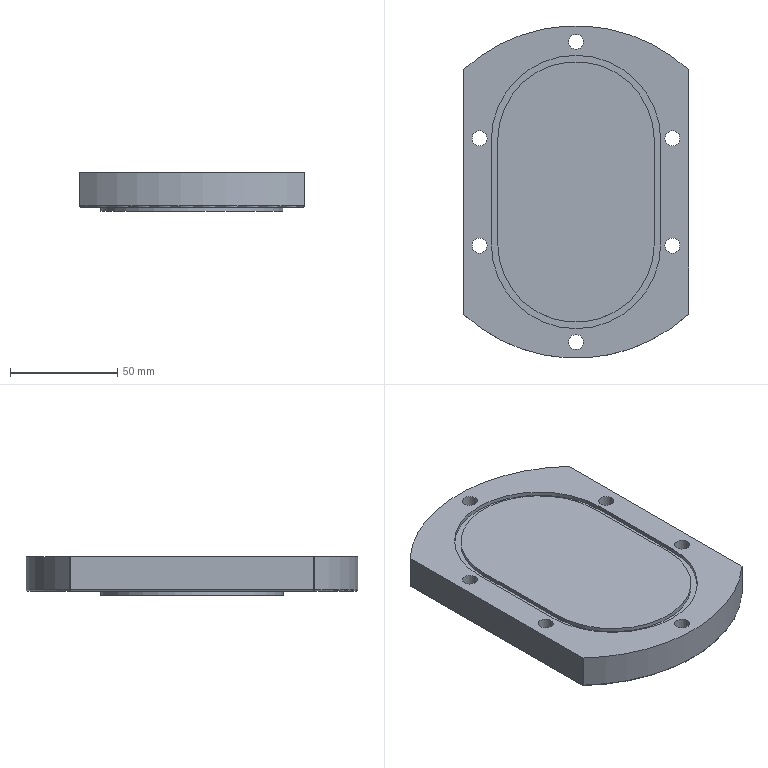NC program | NX | posted with a generic post | part box 105 x 155 x 18 mm
Whole program, first 1635 of 1782 lines:
N10 G17 G21 G94 G90
(FLOOR_WALL_COPY_1 , TOOL : D50)
N12 T02 M6
N14 G54
N16 G17 G0 G90 X-75.614 Y87.319 S1200 M3
N18 G43 Z30. H2
N20 Z7.65
N22 G94 G1 Z4.65 F1000.
N24 X-70.946
N26 X70.941 F2000.
N28 G2 X99.91 Y51.711 R112.241
N30 X101.323 Y48.895 R111.209
N32 X101.458 Y48.614 R111.395
N34 G1 X-101.459
N36 G3 X-109.633 Y25.245 R112.068
N38 X-110.453 Y21.379 R112.313
N40 X-112.069 Y9.909 R112.271
N42 G1 X112.07
N44 G2 X112.486 Y2.175 R112.313
N46 X112.5 Y1.294 R112.271
N48 G1 Y-1.294
N50 G2 X110.453 Y-21.377 R112.271
N52 X109.632 Y-25.245 R112.313
N54 X108.756 Y-28.795 R112.07
N56 G1 X-108.763
N58 G3 X-90.022 Y-67.5 R113.082
N60 G1 X90.002
N62 X93.727
N64 Z7.65
N66 G0 Z30.
N68 X-75.615 Y87.319
N70 Z7.3
N72 G1 Z4.3 F1000.
N74 X-70.946
N76 X70.942 F2000.
N78 G2 X88.734 Y69.167 R112.103
N80 X97.746 Y55.699 R112.241
N82 X101.46 Y48.614 R111.936
N84 G1 X-101.46
N86 G3 X-102.602 Y46.155 R110.938
N88 X-107.9 Y31.856 R112.068
N90 X-109.634 Y25.238 R110.735
N92 X-110.408 Y21.612 R112.347
N94 X-112.069 Y9.909 R112.313
N96 G1 X112.07
N98 G2 X112.5 Y1.291 R112.313
N100 G1 Y-1.284
N102 G2 X110.412 Y-21.592 R112.313
N104 X109.634 Y-25.238 R112.347
N106 X108.757 Y-28.795 R110.742
N108 G1 X-108.755
N110 G3 X-101.989 Y-47.492 R111.212
N112 X-98.21 Y-54.871 R111.831
N114 X-93.788 Y-62.135 R112.247
N116 X-90.007 Y-67.5 R112.235
N118 G1 X90.003
N120 X93.727
N122 Z7.3
N124 G0 Z30.
N126 X-75.621 Y87.319
N128 Z6.95
N130 G1 Z3.95 F1000.
N132 X-70.952
N134 X70.951 F2000.
N136 G2 X94.377 Y61.235 R111.958
N138 X101.461 Y48.614 R111.28
N140 G1 X-101.461
N142 G3 X-102.339 Y46.736 R111.642
N144 X-104.144 Y42.556 R110.938
N146 X-105.517 Y39.02 R111.642
N148 X-107.606 Y32.837 R110.925
N150 X-109.531 Y25.683 R110.735
N152 X-109.633 Y25.245 R110.925
N154 X-110.481 Y21.234 R112.352
N156 X-112.068 Y9.909 R112.347
N158 G1 X112.069
N160 G2 X112.5 Y1.217 R112.347
N162 G1 Y-1.212
N164 G2 X110.511 Y-21.078 R112.347
N166 X109.633 Y-25.245 R112.351
N168 X109.534 Y-25.671 R110.932
N170 X108.757 Y-28.795 R110.742
N172 G1 X-108.755
N174 G3 X-107.927 Y-31.763 R110.883
N176 X-102.013 Y-47.442 R111.831
N178 X-98.213 Y-54.866 R110.045
N180 X-90.014 Y-67.5 R112.024
N182 G1 X90.009
N184 X93.73
N186 Z6.95
N188 G0 Z30.
N190 X-75.629 Y87.319
N192 Z6.6
N194 G1 Z3.6 F1000.
N196 X-70.96
N198 X70.955 F2000.
N200 G2 X95.056 Y60.179 R111.788
N202 X101.461 Y48.614 R111.28
N204 G1 X-101.467
N206 G3 X-107.823 Y32.116 R111.531
N208 X-109.474 Y25.926 R110.925
N210 X-112.074 Y9.909 R112.101
N212 G1 X112.073
N214 G2 X112.5 Y1.638 R112.103
N216 G1 Y-1.65
N218 G2 X109.476 Y-25.921 R112.103
N220 X108.757 Y-28.795 R110.932
N222 G1 X-108.756
N224 G3 X-102.23 Y-46.972 R111.909
N226 X-98.213 Y-54.866 R110.045
N228 X-90.014 Y-67.5 R112.024
N230 G1 X90.011
N232 X93.731
N234 Z6.6
N236 G0 Z30.
N238 X-75.653 Y87.297
N240 Z6.25
N242 G1 Z3.25 F1000.
N244 X-70.986
N246 X70.981 F2000.
N248 G2 X93.922 Y61.939 R111.788
N250 X98.532 Y54.299 R110.498
N252 X101.468 Y48.598 R112.024
N254 G1 X-101.475
N256 G3 X-104.906 Y40.665 R111.531
N258 X-107.813 Y32.15 R111.134
N260 X-108.774 Y28.712 R111.531
N262 X-109.386 Y26.294 R112.101
N264 X-112.077 Y9.899 R112.004
N266 G1 X112.075
N268 G2 X112.5 Y1.781 R112.006
N270 G1 Y-1.798
N272 G2 X109.384 Y-26.302 R112.006
N274 X108.774 Y-28.712 R112.103
N276 G1 X108.751 Y-28.801
N278 X-108.755
N280 G3 X-101.738 Y-48.027 R111.459
N282 X-98.21 Y-54.872 R111.909
N284 G1 X-98.144 Y-54.99
N286 G3 X-92.27 Y-64.37 R109.794
N288 X-90.007 Y-67.5 R112.274
N290 G1 X90.011
N292 X93.731
N294 Z6.25
N296 G0 Z30.
N298 X-75.638 Y87.294
N300 Z5.9
N302 G1 Z2.9 F1000.
N304 X-70.971
N306 X70.971 F2000.
N308 G2 X85.956 Y72.586 R112.036
N310 X91.507 Y65.449 R112.37
N312 X99.844 Y51.84 R110.498
N314 X101.467 Y48.596 R111.457
N316 G1 X-101.474
N318 G3 X-108.753 Y28.792 R111.134
N320 X-109.187 Y27.106 R112.004
N322 X-112.078 Y9.897 R111.966
N324 G1 X112.076
N326 G2 X112.5 Y1.834 R111.968
N328 G1 Y-1.853
N330 G2 X109.189 Y-27.099 R111.968
N332 X108.75 Y-28.801 R112.006
N334 G1 X-108.755
N336 G3 X-90.006 Y-67.5 R113.109
N338 G1 X90.003
N340 X93.727
N342 Z5.9
N344 G0 Z30.
N346 X-75.632 Y87.301
N348 Z5.55
N350 G1 Z2.55 F1000.
N352 X-70.966
N354 X70.962 F2000.
N356 G2 X98.163 Y54.958 R112.284
N358 X99.878 Y51.773 R112.37
N360 X101.464 Y48.601 R111.357
N362 G1 X-101.47
N364 G3 X-107.634 Y32.745 R111.273
N366 X-109.35 Y26.445 R112.1
N368 X-112.078 Y9.9 R111.966
N370 G1 X112.076
N372 G2 X112.5 Y1.834 R111.968
N374 G1 Y-1.853
N376 G2 X109.35 Y-26.443 R111.968
N378 X108.754 Y-28.8 R112.102
N380 G1 X-108.762
N382 G3 X-90.006 Y-67.5 R112.72
N384 G1 X90.003
N386 X93.727
N388 Z5.55
N390 G0 Z30.
N392 X-75.631 Y87.302
N394 Z5.2
N396 G1 Z2.2 F1000.
N398 X-70.965
N400 X70.961 F2000.
N402 G2 X101.464 Y48.601 R112.412
N404 G1 X-101.472
N406 G3 X-107.864 Y31.977 R110.937
N408 X-109.348 Y26.452 R112.1
N410 X-112.079 Y9.901 R111.905
N412 G1 X112.077
N414 G2 X112.5 Y1.915 R111.908
N416 G1 Y-1.937
N418 G2 X109.349 Y-26.448 R111.908
N420 X108.754 Y-28.8 R112.102
N422 G1 X-108.762
N424 G3 X-101.44 Y-48.651 R111.402
N426 X-100.103 Y-51.337 R111.147
N428 X-99.926 Y-51.68 R111.402
N430 G1 X-98.201 Y-54.887
N432 G3 X-98.078 Y-55.108 R112.256
N434 X-90.006 Y-67.5 R112.252
N436 G1 X90.002
N438 X93.727
N440 Z5.2
N442 G0 Z30.
N444 X-75.632 Y87.302
N446 Z4.85
N448 G1 Z1.85 F1000.
N450 X-70.965
N452 X70.961 F2000.
N454 G2 X98.468 Y54.41 R112.27
N456 X99.921 Y51.69 R112.297
N458 X101.325 Y48.889 R111.102
N460 X101.464 Y48.601 R111.145
N462 G1 X-101.472
N464 G3 X-107.772 Y32.289 R110.937
N466 X-109.377 Y26.333 R112.065
N468 X-112.079 Y9.901 R111.905
N470 G1 X112.077
N472 G2 X112.5 Y1.915 R111.908
N474 G1 Y-1.937
N476 G2 X109.378 Y-26.329 R111.908
N478 X108.755 Y-28.8 R112.067
N480 G1 X-108.756
N482 G3 X-90.007 Y-67.5 R112.605
N484 G1 X90.002
N486 X93.727
N488 Z4.85
N490 G0 Z30.
N492 X-75.615 Y87.319
N494 Z4.5
N496 G1 Z1.5 F1000.
N498 X-70.947
N500 X70.942 F2000.
N502 G2 X92.898 Y63.46 R112.082
N504 X97.478 Y56.165 R112.297
N506 X101.46 Y48.614 R111.937
N508 G1 X-101.459
N510 G3 X-108.239 Y30.685 R112.065
N512 X-109.635 Y25.237 R112.103
N514 X-110.409 Y21.604 R112.345
N516 X-112.069 Y9.909 R112.311
N518 G1 X112.07
N520 G2 X112.5 Y1.296 R112.311
N522 G1 Y-1.288
N524 G2 X110.409 Y-21.605 R112.311
N526 X109.635 Y-25.237 R112.346
N528 X108.756 Y-28.795 R112.105
N530 G1 X-108.755
N532 G3 X-101.856 Y-47.777 R111.107
N534 X-98.21 Y-54.872 R111.838
N536 X-93.852 Y-62.039 R112.245
N538 X-90.007 Y-67.5 R112.234
N540 G1 X90.003
N542 X93.727
N544 Z4.5
N546 G0 Z30.
N548 X-75.621 Y87.319
N550 Z4.15
N552 G1 Z1.15 F1000.
N554 X-70.952
N556 X70.95 F2000.
N558 G2 X94.377 Y61.236 R111.982
N560 X101.461 Y48.614 R111.309
N562 G1 X-101.46
N564 G3 X-102.512 Y46.353 R111.74
N566 X-107.911 Y31.819 R112.103
N568 X-109.633 Y25.244 R110.994
N570 X-110.47 Y21.29 R112.352
N572 X-112.068 Y9.909 R112.346
N574 G1 X112.069
N576 G2 X112.5 Y1.22 R112.346
N578 G1 Y-1.214
N580 G2 X110.505 Y-21.112 R112.346
N582 X109.633 Y-25.244 R112.351
N584 X108.756 Y-28.795 R111.001
N586 G1 X-108.755
N588 G3 X-107.859 Y-31.994 R110.902
N590 X-102.027 Y-47.411 R111.838
N592 X-98.213 Y-54.867 R110.088
N594 X-90.014 Y-67.5 R112.029
N596 G1 X90.009
N598 X93.73
N600 Z4.15
N602 G0 Z30.
N604 X-75.621 Y87.319
N606 Z3.8
N608 G1 Z0.8 F1000.
N610 X-70.952
N612 X70.95 F2000.
N614 G2 X93.525 Y62.532 R111.982
N616 X94.878 Y60.458 R112.368
N618 X101.461 Y48.614 R111.309
N620 G1 X-101.463
N622 G3 X-104.199 Y42.422 R111.661
N624 X-105.527 Y38.993 R111.74
N626 X-107.477 Y33.254 R110.994
N628 X-112.076 Y9.909 R112.194
N630 G1 X112.073
N632 G2 X112.5 Y1.68 R112.195
N634 G1 Y-1.718
N636 G2 X108.76 Y-28.795 R112.195
N638 G1 X-108.757
N640 G3 X-102.086 Y-47.284 R111.642
N642 X-98.213 Y-54.867 R110.088
N644 X-90.014 Y-67.5 R112.029
N646 G1 X90.009
N648 X93.73
N650 Z3.8
N652 G0 Z30.
N654 X-75.644 Y87.297
N656 Z3.45
N658 G1 Z0.45 F1000.
N660 X-70.973
N662 X70.981 F2000.
N664 G2 X88.117 Y69.95 R111.495
N666 X92.269 Y64.372 R112.368
N668 X99.593 Y52.321 R110.523
N670 X99.795 Y51.936 R112.368
N672 X101.466 Y48.598 R111.644
N674 G1 X-101.476
N676 G3 X-107.724 Y32.448 R111.462
N678 X-112.077 Y9.899 R112.194
N680 G1 X112.075
N682 G2 X112.5 Y1.771 R112.018
N684 G1 Y-1.788
N686 G2 X112.204 Y-8.333 R112.018
N688 X108.758 Y-28.801 R112.195
N690 G1 X-108.755
N692 G3 X-90.007 Y-67.5 R112.76
N694 G1 X90.011
N696 X93.731
N698 Z3.45
N700 G0 Z30.
N702 X-75.649 Y87.293
N704 Z3.1
N706 G1 Z0.1 F1000.
N708 X-70.978
N710 X70.986 F2000.
N712 G2 X88.748 Y69.145 R111.495
N714 X91.643 Y65.258 R112.395
N716 X99.837 Y51.853 R110.523
N718 X101.467 Y48.595 R111.474
N720 G1 X-101.477
N722 G3 X-108.761 Y28.76 R111.462
N724 X-109.934 Y23.91 R112.015
N726 X-112.078 Y9.896 R111.977
N728 G1 X112.076
N730 G2 X112.5 Y1.819 R111.979
N732 G1 Y-1.837
N734 G2 X109.904 Y-24.051 R111.979
N736 X108.75 Y-28.802 R112.018
N738 G1 X-108.755
N740 G3 X-90.006 Y-67.5 R113.105
N742 G1 X90.011
N744 X93.731
N746 Z3.1
N748 G0 Z30.
(FLOOR_WALL_COPY_COPY , TOOL : D50)
N750 X-75.612 Y87.319 S2500
N752 Z3.
N754 G1 Z0. F1000.
N756 X-70.944
N758 X70.94
N760 G2 X99.927 Y51.677 R112.283
N762 X101.311 Y48.918 R111.144
N764 X101.458 Y48.614 R111.395
N766 G1 X-101.459
N768 G3 X-109.634 Y25.24 R112.055
N770 X-112.077 Y9.909 R111.876
N772 G1 X112.076
N774 G2 X112.5 Y1.904 R111.879
N776 G1 Y-1.918
N778 G2 X109.634 Y-25.24 R111.879
N780 X108.756 Y-28.795 R112.057
N782 G1 X-108.763
N784 G3 X-90.022 Y-67.5 R113.084
N786 G1 X90.002
N788 X93.727
N790 Z3.
N792 G0 Z30.
N794 M5
(DRILLING , TOOL : ZXZ)
N796 T01 M6
N798 G54
N800 G17 G0 G90 X70. Y0. S5000 M3
N802 G43 Z30. H1
N804 G94 G81 G98 Z-1. F250. R3.
N806 X25. Y-45.
N808 X-25.
N810 X-70. Y0.
N812 X-25. Y45.
N814 X25.
N816 G80
N818 G0 X25. Y45. Z30.
N820 M5
(DRILLING_COPY , TOOL : 7.0ZT)
N822 T09 M6
N824 G54
N826 G17 G0 G90 X70. Y0. S2000 M3
N828 G43 Z30. H9
N830 G94 G83 G98 Z-21.103 F200. Q2. R3.
N832 X25. Y-45.
N834 Y45.
N836 X-25.
N838 Y-45.
N840 X-70. Y0.
N842 G80
N844 G0 X-70. Y0. Z30.
N846 M5
(PLANAR_PROFILE , TOOL : D3)
N848 T03 M6
N850 G54
N852 G17 G0 G90 X0. Y38. S5000 M3
N854 G43 Z30. H3
N856 Z3.
N858 G94 G1 Z-0.05 F500.
N860 X-24.25 F1100.
N862 G3 X-62.25 Y0. R38.
N864 X-24.25 Y-38. R38.
N866 G1 X24.25
N868 G3 X62.25 Y0. R38.
N870 X24.25 Y38. R38.
N872 G1 X0.
N874 Z2.95
N876 Z-0.1 F500.
N878 X24.25 F1100.
N880 G2 X62.25 Y0. R38.
N882 X24.25 Y-38. R38.
N884 G1 X-24.25
N886 G2 X-62.25 Y0. R38.
N888 X-24.25 Y38. R38.
N890 G1 X0.
N892 Z2.9
N894 Z-0.15 F500.
N896 X-24.25 F1100.
N898 G3 X-62.25 Y0. R38.
N900 X-24.25 Y-38. R38.
N902 G1 X24.25
N904 G3 X62.25 Y0. R38.
N906 X24.25 Y38. R38.
N908 G1 X0.
N910 Z2.85
N912 Z-0.2 F500.
N914 X24.25 F1100.
N916 G2 X62.25 Y0. R38.
N918 X24.25 Y-38. R38.
N920 G1 X-24.25
N922 G2 X-62.25 Y0. R38.
N924 X-24.25 Y38. R38.
N926 G1 X0.
N928 Z2.8
N930 Z-0.25 F500.
N932 X-24.25 F1100.
N934 G3 X-62.25 Y0. R38.
N936 X-24.25 Y-38. R38.
N938 G1 X24.25
N940 G3 X62.25 Y0. R38.
N942 X24.25 Y38. R38.
N944 G1 X0.
N946 Z2.75
N948 Z-0.3 F500.
N950 X24.25 F1100.
N952 G2 X62.25 Y0. R38.
N954 X24.25 Y-38. R38.
N956 G1 X-24.25
N958 G2 X-62.25 Y0. R38.
N960 X-24.25 Y38. R38.
N962 G1 X0.
N964 Z2.7
N966 Z-0.35 F500.
N968 X-24.25 F1100.
N970 G3 X-62.25 Y0. R38.
N972 X-24.25 Y-38. R38.
N974 G1 X24.25
N976 G3 X62.25 Y0. R38.
N978 X24.25 Y38. R38.
N980 G1 X0.
N982 Z2.65
N984 Z-0.4 F500.
N986 X24.25 F1100.
N988 G2 X62.25 Y0. R38.
N990 X24.25 Y-38. R38.
N992 G1 X-24.25
N994 G2 X-62.25 Y0. R38.
N996 X-24.25 Y38. R38.
N998 G1 X0.
N1000 Z2.6
N1002 Z-0.45 F500.
N1004 X-24.25 F1100.
N1006 G3 X-62.25 Y0. R38.
N1008 X-24.25 Y-38. R38.
N1010 G1 X24.25
N1012 G3 X62.25 Y0. R38.
N1014 X24.25 Y38. R38.
N1016 G1 X0.
N1018 Z2.55
N1020 Z-0.5 F500.
N1022 X24.25 F1100.
N1024 G2 X62.25 Y0. R38.
N1026 X24.25 Y-38. R38.
N1028 G1 X-24.25
N1030 G2 X-62.25 Y0. R38.
N1032 X-24.25 Y38. R38.
N1034 G1 X0.
N1036 Z2.5
N1038 Z-0.55 F500.
N1040 X-24.25 F1100.
N1042 G3 X-62.25 Y0. R38.
N1044 X-24.25 Y-38. R38.
N1046 G1 X24.25
N1048 G3 X62.25 Y0. R38.
N1050 X24.25 Y38. R38.
N1052 G1 X0.
N1054 Z2.45
N1056 Z-0.6 F500.
N1058 X24.25 F1100.
N1060 G2 X62.25 Y0. R38.
N1062 X24.25 Y-38. R38.
N1064 G1 X-24.25
N1066 G2 X-62.25 Y0. R38.
N1068 X-24.25 Y38. R38.
N1070 G1 X0.
N1072 Z2.4
N1074 Z-0.65 F500.
N1076 X-24.25 F1100.
N1078 G3 X-62.25 Y0. R38.
N1080 X-24.25 Y-38. R38.
N1082 G1 X24.25
N1084 G3 X62.25 Y0. R38.
N1086 X24.25 Y38. R38.
N1088 G1 X0.
N1090 Z2.35
N1092 Z-0.7 F500.
N1094 X24.25 F1100.
N1096 G2 X62.25 Y0. R38.
N1098 X24.25 Y-38. R38.
N1100 G1 X-24.25
N1102 G2 X-62.25 Y0. R38.
N1104 X-24.25 Y38. R38.
N1106 G1 X0.
N1108 Z2.3
N1110 Z-0.75 F500.
N1112 X-24.25 F1100.
N1114 G3 X-62.25 Y0. R38.
N1116 X-24.25 Y-38. R38.
N1118 G1 X24.25
N1120 G3 X62.25 Y0. R38.
N1122 X24.25 Y38. R38.
N1124 G1 X0.
N1126 Z2.25
N1128 Z-0.8 F500.
N1130 X24.25 F1100.
N1132 G2 X62.25 Y0. R38.
N1134 X24.25 Y-38. R38.
N1136 G1 X-24.25
N1138 G2 X-62.25 Y0. R38.
N1140 X-24.25 Y38. R38.
N1142 G1 X0.
N1144 Z2.2
N1146 Z-0.85 F500.
N1148 X-24.25 F1100.
N1150 G3 X-62.25 Y0. R38.
N1152 X-24.25 Y-38. R38.
N1154 G1 X24.25
N1156 G3 X62.25 Y0. R38.
N1158 X24.25 Y38. R38.
N1160 G1 X0.
N1162 Z2.15
N1164 Z-0.9 F500.
N1166 X24.25 F1100.
N1168 G2 X62.25 Y0. R38.
N1170 X24.25 Y-38. R38.
N1172 G1 X-24.25
N1174 G2 X-62.25 Y0. R38.
N1176 X-24.25 Y38. R38.
N1178 G1 X0.
N1180 Z2.1
N1182 Z-0.95 F500.
N1184 X-24.25 F1100.
N1186 G3 X-62.25 Y0. R38.
N1188 X-24.25 Y-38. R38.
N1190 G1 X24.25
N1192 G3 X62.25 Y0. R38.
N1194 X24.25 Y38. R38.
N1196 G1 X0.
N1198 Z2.05
N1200 Z-1. F500.
N1202 X24.25 F1100.
N1204 G2 X62.25 Y0. R38.
N1206 X24.25 Y-38. R38.
N1208 G1 X-24.25
N1210 G2 X-62.25 Y0. R38.
N1212 X-24.25 Y38. R38.
N1214 G1 X0.
N1216 Z2.
N1218 Z-1.05 F500.
N1220 X-24.25 F1100.
N1222 G3 X-62.25 Y0. R38.
N1224 X-24.25 Y-38. R38.
N1226 G1 X24.25
N1228 G3 X62.25 Y0. R38.
N1230 X24.25 Y38. R38.
N1232 G1 X0.
N1234 Z1.95
N1236 Z-1.1 F500.
N1238 X24.25 F1100.
N1240 G2 X62.25 Y0. R38.
N1242 X24.25 Y-38. R38.
N1244 G1 X-24.25
N1246 G2 X-62.25 Y0. R38.
N1248 X-24.25 Y38. R38.
N1250 G1 X0.
N1252 Z1.9
N1254 Z-1.15 F500.
N1256 X-24.25 F1100.
N1258 G3 X-62.25 Y0. R38.
N1260 X-24.25 Y-38. R38.
N1262 G1 X24.25
N1264 G3 X62.25 Y0. R38.
N1266 X24.25 Y38. R38.
N1268 G1 X0.
N1270 Z1.85
N1272 Z-1.2 F500.
N1274 X24.25 F1100.
N1276 G2 X62.25 Y0. R38.
N1278 X24.25 Y-38. R38.
N1280 G1 X-24.25
N1282 G2 X-62.25 Y0. R38.
N1284 X-24.25 Y38. R38.
N1286 G1 X0.
N1288 Z1.8
N1290 Z-1.25 F500.
N1292 X-24.25 F1100.
N1294 G3 X-62.25 Y0. R38.
N1296 X-24.25 Y-38. R38.
N1298 G1 X24.25
N1300 G3 X62.25 Y0. R38.
N1302 X24.25 Y38. R38.
N1304 G1 X0.
N1306 Z1.75
N1308 Z-1.3 F500.
N1310 X24.25 F1100.
N1312 G2 X62.25 Y0. R38.
N1314 X24.25 Y-38. R38.
N1316 G1 X-24.25
N1318 G2 X-62.25 Y0. R38.
N1320 X-24.25 Y38. R38.
N1322 G1 X0.
N1324 Z1.7
N1326 Z-1.35 F500.
N1328 X-24.25 F1100.
N1330 G3 X-62.25 Y0. R38.
N1332 X-24.25 Y-38. R38.
N1334 G1 X24.25
N1336 G3 X62.25 Y0. R38.
N1338 X24.25 Y38. R38.
N1340 G1 X0.
N1342 Z1.65
N1344 Z-1.4 F500.
N1346 X24.25 F1100.
N1348 G2 X62.25 Y0. R38.
N1350 X24.25 Y-38. R38.
N1352 G1 X-24.25
N1354 G2 X-62.25 Y0. R38.
N1356 X-24.25 Y38. R38.
N1358 G1 X0.
N1360 Z1.6
N1362 Z-1.45 F500.
N1364 X-24.25 F1100.
N1366 G3 X-62.25 Y0. R38.
N1368 X-24.25 Y-38. R38.
N1370 G1 X24.25
N1372 G3 X62.25 Y0. R38.
N1374 X24.25 Y38. R38.
N1376 G1 X0.
N1378 Z1.55
N1380 Z-1.5 F500.
N1382 X24.25 F1100.
N1384 G2 X62.25 Y0. R38.
N1386 X24.25 Y-38. R38.
N1388 G1 X-24.25
N1390 G2 X-62.25 Y0. R38.
N1392 X-24.25 Y38. R38.
N1394 G1 X0.
N1396 Z1.5
N1398 Z-1.55 F500.
N1400 X-24.25 F1100.
N1402 G3 X-62.25 Y0. R38.
N1404 X-24.25 Y-38. R38.
N1406 G1 X24.25
N1408 G3 X62.25 Y0. R38.
N1410 X24.25 Y38. R38.
N1412 G1 X0.
N1414 Z1.45
N1416 Z-1.6 F500.
N1418 X24.25 F1100.
N1420 G2 X62.25 Y0. R38.
N1422 X24.25 Y-38. R38.
N1424 G1 X-24.25
N1426 G2 X-62.25 Y0. R38.
N1428 X-24.25 Y38. R38.
N1430 G1 X0.
N1432 Z1.4
N1434 Z-1.65 F500.
N1436 X-24.25 F1100.
N1438 G3 X-62.25 Y0. R38.
N1440 X-24.25 Y-38. R38.
N1442 G1 X24.25
N1444 G3 X62.25 Y0. R38.
N1446 X24.25 Y38. R38.
N1448 G1 X0.
N1450 Z1.35
N1452 Z-1.7 F500.
N1454 X24.25 F1100.
N1456 G2 X62.25 Y0. R38.
N1458 X24.25 Y-38. R38.
N1460 G1 X-24.25
N1462 G2 X-62.25 Y0. R38.
N1464 X-24.25 Y38. R38.
N1466 G1 X0.
N1468 Z1.3
N1470 Z-1.75 F500.
N1472 X-24.25 F1100.
N1474 G3 X-62.25 Y0. R38.
N1476 X-24.25 Y-38. R38.
N1478 G1 X24.25
N1480 G3 X62.25 Y0. R38.
N1482 X24.25 Y38. R38.
N1484 G1 X0.
N1486 Z1.25
N1488 Z-1.8 F500.
N1490 X24.25 F1100.
N1492 G2 X62.25 Y0. R38.
N1494 X24.25 Y-38. R38.
N1496 G1 X-24.25
N1498 G2 X-62.25 Y0. R38.
N1500 X-24.25 Y38. R38.
N1502 G1 X0.
N1504 Z1.2
N1506 G0 Z30.
N1508 M5
(ZLEVEL_PROFILE_COPY , TOOL : D25R0.5)
N1510 T05 M6
N1512 G54
N1514 G17 G0 G90 X-65.122 Y74.248 S2000 M3
N1516 G43 Z30. H5
N1518 Z-0.348
N1520 G94 G1 X-60.623 Y66.405 F1000.
N1522 G3 X-58.461 Y65.149 R2.5
N1524 G1 X-57.852 Y65.147 F2200.
N1526 X-56.741 Y65.15
N1528 X56.81 Y65.149
N1530 X57.852 Y65.147
N1532 X58.461 Y65.149
N1534 G3 X60.623 Y66.405 R2.5
N1536 G1 X65.122 Y74.248
N1538 X-65.09 Y74.257 Z-0.696
N1540 X-60.619 Y66.411 F1000.
N1542 G3 X-58.461 Y65.149 R2.5
N1544 G1 X-57.243 Y65.142 F2200.
N1546 G2 X-56.789 Y65.15 R13.15
N1548 G1 X56.831
N1550 G2 X57.243 Y65.142 R13.15
N1552 G1 X58.461 Y65.149
N1554 G3 X60.619 Y66.411 R2.5
N1556 G1 X65.09 Y74.257
N1558 X-65.09 Z-1.043
N1560 X-60.619 Y66.411 F1000.
N1562 G3 X-58.461 Y65.149 R2.5
N1564 G1 X-57.243 Y65.142 F2200.
N1566 G2 X-56.789 Y65.15 R13.15
N1568 G1 X56.831
N1570 G2 X57.243 Y65.142 R13.15
N1572 G1 X58.461 Y65.149
N1574 G3 X60.619 Y66.411 R2.5
N1576 G1 X65.09 Y74.257
N1578 X-65.09 Z-1.391
N1580 X-60.619 Y66.411 F1000.
N1582 G3 X-58.461 Y65.149 R2.5
N1584 G1 X-57.243 Y65.142 F2200.
N1586 G2 X-56.789 Y65.15 R13.15
N1588 G1 X56.831
N1590 G2 X57.243 Y65.142 R13.15
N1592 G1 X58.461 Y65.149
N1594 G3 X60.619 Y66.411 R2.5
N1596 G1 X65.09 Y74.257
N1598 X-65.09 Z-1.739
N1600 X-60.619 Y66.411 F1000.
N1602 G3 X-58.461 Y65.149 R2.5
N1604 G1 X-57.243 Y65.142 F2200.
N1606 G2 X-56.789 Y65.15 R13.15
N1608 G1 X56.831
N1610 G2 X57.243 Y65.142 R13.15
N1612 G1 X58.461 Y65.149
N1614 G3 X60.619 Y66.411 R2.5
N1616 G1 X65.09 Y74.257
N1618 X-65.089 Z-2.087
N1620 X-60.619 Y66.411 F1000.
N1622 G3 X-58.461 Y65.149 R2.5
N1624 G1 X-57.243 Y65.142 F2200.
N1626 G2 X-56.789 Y65.15 R13.15
N1628 G1 X56.831
N1630 G2 X57.243 Y65.142 R13.15
N1632 G1 X58.461 Y65.149
N1634 G3 X60.619 Y66.411 R2.5
N1636 G1 X65.089 Y74.257
N1638 X-65.089 Z-2.435
N1640 X-60.619 Y66.412 F1000.
N1642 G3 X-58.461 Y65.149 R2.5
N1644 G1 X-57.243 Y65.142 F2200.
N1646 G2 X-56.789 Y65.15 R13.15
N1648 G1 X56.831
N1650 G2 X57.243 Y65.142 R13.15
N1652 G1 X58.461 Y65.149
N1654 G3 X60.619 Y66.412 R2.5
N1656 G1 X65.089 Y74.257
N1658 X-65.089 Z-2.783
N1660 X-60.619 Y66.412 F1000.
N1662 G3 X-58.461 Y65.149 R2.5
N1664 G1 X-57.243 Y65.142 F2200.
N1666 G2 X-56.789 Y65.15 R13.15
N1668 G1 X56.831
N1670 G2 X57.243 Y65.142 R13.15
N1672 G1 X58.461 Y65.149
N1674 G3 X60.619 Y66.412 R2.5
N1676 G1 X65.089 Y74.257
N1678 X-65.089 Z-3.13
N1680 X-60.619 Y66.412 F1000.
N1682 G3 X-58.461 Y65.149 R2.5
N1684 G1 X-57.243 Y65.142 F2200.
N1686 G2 X-56.789 Y65.15 R13.15
N1688 G1 X56.831
N1690 G2 X57.243 Y65.142 R13.15
N1692 G1 X58.461 Y65.149
N1694 G3 X60.619 Y66.412 R2.5
N1696 G1 X65.089 Y74.257
N1698 X-65.089 Y74.258 Z-3.478
N1700 X-60.619 Y66.412 F1000.
N1702 G3 X-58.461 Y65.149 R2.5
N1704 G1 X-57.243 Y65.142 F2200.
N1706 G2 X-56.789 Y65.15 R13.15
N1708 G1 X56.831
N1710 G2 X57.243 Y65.142 R13.15
N1712 G1 X58.461 Y65.149
N1714 G3 X60.619 Y66.412 R2.5
N1716 G1 X65.089 Y74.258
N1718 X-65.089 Z-3.826
N1720 X-60.619 Y66.412 F1000.
N1722 G3 X-58.461 Y65.149 R2.5
N1724 G1 X-57.243 Y65.142 F2200.
N1726 G2 X-56.789 Y65.15 R13.15
N1728 G1 X56.831
N1730 G2 X57.243 Y65.142 R13.15
N1732 G1 X58.461 Y65.149
N1734 G3 X60.619 Y66.412 R2.5
N1736 G1 X65.089 Y74.258
N1738 X-65.089 Z-4.174
N1740 X-60.619 Y66.412 F1000.
N1742 G3 X-58.461 Y65.149 R2.5
N1744 G1 X-57.243 Y65.142 F2200.
N1746 G2 X-56.789 Y65.15 R13.15
N1748 G1 X56.831
N1750 G2 X57.243 Y65.142 R13.15
N1752 G1 X58.461 Y65.149
N1754 G3 X60.619 Y66.412 R2.5
N1756 G1 X65.089 Y74.258
N1758 X-65.089 Z-4.522
N1760 X-60.619 Y66.412 F1000.
N1762 G3 X-58.461 Y65.149 R2.5
N1764 G1 X-57.243 Y65.142 F2200.
N1766 G2 X-56.789 Y65.15 R13.15
N1768 G1 X56.831
N1770 G2 X57.243 Y65.142 R13.15
N1772 G1 X58.461 Y65.149
N1774 G3 X60.619 Y66.412 R2.5
N1776 G1 X65.089 Y74.258
N1778 X-65.088 Z-4.87
N1780 X-60.619 Y66.412 F1000.
N1782 G3 X-58.461 Y65.149 R2.5
N1784 G1 X-57.243 Y65.142 F2200.
N1786 G2 X-56.789 Y65.15 R13.15
N1788 G1 X56.831
N1790 G2 X57.243 Y65.142 R13.15
N1792 G1 X58.461 Y65.149
N1794 G3 X60.619 Y66.412 R2.5
N1796 G1 X65.088 Y74.258
N1798 X-65.088 Z-5.217
N1800 X-60.619 Y66.412 F1000.
N1802 G3 X-58.461 Y65.149 R2.5
N1804 G1 X-57.243 Y65.142 F2200.
N1806 G2 X-56.789 Y65.15 R13.15
N1808 G1 X56.831
N1810 G2 X57.243 Y65.142 R13.15
N1812 G1 X58.461 Y65.149
N1814 G3 X60.619 Y66.412 R2.5
N1816 G1 X65.088 Y74.258
N1818 X-65.088 Z-5.565
N1820 X-60.619 Y66.412 F1000.
N1822 G3 X-58.461 Y65.149 R2.5
N1824 G1 X-57.243 Y65.142 F2200.
N1826 G2 X-56.789 Y65.15 R13.15
N1828 G1 X56.831
N1830 G2 X57.243 Y65.142 R13.15
N1832 G1 X58.461 Y65.149
N1834 G3 X60.619 Y66.412 R2.5
N1836 G1 X65.088 Y74.258
N1838 X-65.088 Z-5.913
N1840 X-60.619 Y66.412 F1000.
N1842 G3 X-58.461 Y65.149 R2.5
N1844 G1 X-57.243 Y65.142 F2200.
N1846 G2 X-56.789 Y65.15 R13.15
N1848 G1 X56.831
N1850 G2 X57.243 Y65.142 R13.15
N1852 G1 X58.461 Y65.149
N1854 G3 X60.619 Y66.412 R2.5
N1856 G1 X65.088 Y74.258
N1858 X-65.088 Z-6.261
N1860 X-60.619 Y66.412 F1000.
N1862 G3 X-58.461 Y65.149 R2.5
N1864 G1 X-57.243 Y65.142 F2200.
N1866 G2 X-56.789 Y65.15 R13.15
N1868 G1 X56.831
N1870 G2 X57.243 Y65.142 R13.15
N1872 G1 X58.461 Y65.149
N1874 G3 X60.619 Y66.412 R2.5
N1876 G1 X65.088 Y74.258
N1878 X-65.088 Z-6.609
N1880 X-60.619 Y66.412 F1000.
N1882 G3 X-58.461 Y65.149 R2.5
N1884 G1 X-57.243 Y65.142 F2200.
N1886 G2 X-56.789 Y65.15 R13.15
N1888 G1 X56.831
N1890 G2 X57.243 Y65.142 R13.15
N1892 G1 X58.461 Y65.149
N1894 G3 X60.619 Y66.412 R2.5
N1896 G1 X65.088 Y74.258
N1898 X-65.088 Z-6.957
N1900 X-60.619 Y66.412 F1000.
N1902 G3 X-58.461 Y65.149 R2.5
N1904 G1 X-57.243 Y65.142 F2200.
N1906 G2 X-56.789 Y65.15 R13.15
N1908 G1 X56.831
N1910 G2 X57.243 Y65.142 R13.15
N1912 G1 X58.461 Y65.149
N1914 G3 X60.619 Y66.412 R2.5
N1916 G1 X65.088 Y74.258
N1918 X-65.088 Z-7.304
N1920 X-60.619 Y66.412 F1000.
N1922 G3 X-58.461 Y65.149 R2.5
N1924 G1 X-57.243 Y65.142 F2200.
N1926 G2 X-56.789 Y65.15 R13.15
N1928 G1 X56.831
N1930 G2 X57.243 Y65.142 R13.15
N1932 G1 X58.461 Y65.149
N1934 G3 X60.619 Y66.412 R2.5
N1936 G1 X65.088 Y74.258
N1938 X-65.087 Z-7.652
N1940 X-60.619 Y66.412 F1000.
N1942 G3 X-58.461 Y65.149 R2.5
N1944 G1 X-57.243 Y65.142 F2200.
N1946 G2 X-56.789 Y65.15 R13.15
N1948 G1 X56.831
N1950 G2 X57.243 Y65.142 R13.15
N1952 G1 X58.461 Y65.149
N1954 G3 X60.619 Y66.412 R2.5
N1956 G1 X65.087 Y74.258
N1958 X-65.087 Z-8.
N1960 X-60.619 Y66.412 F1000.
N1962 G3 X-58.461 Y65.149 R2.5
N1964 G1 X-57.243 Y65.142 F2200.
N1966 G2 X-56.789 Y65.15 R13.15
N1968 G1 X56.831
N1970 G2 X57.243 Y65.142 R13.15
N1972 G1 X58.461 Y65.149
N1974 G3 X60.619 Y66.412 R2.5
N1976 G1 X65.087 Y74.258
N1978 X-65.087 Z-8.348
N1980 X-60.619 Y66.412 F1000.
N1982 G3 X-58.461 Y65.149 R2.5
N1984 G1 X-57.243 Y65.142 F2200.
N1986 G2 X-56.789 Y65.15 R13.15
N1988 G1 X56.831
N1990 G2 X57.243 Y65.142 R13.15
N1992 G1 X58.461 Y65.149
N1994 G3 X60.619 Y66.412 R2.5
N1996 G1 X65.087 Y74.258
N1998 X-65.087 Z-8.696
N2000 X-60.619 Y66.412 F1000.
N2002 G3 X-58.461 Y65.149 R2.5
N2004 G1 X-57.243 Y65.142 F2200.
N2006 G2 X-56.789 Y65.15 R13.15
N2008 G1 X56.831
N2010 G2 X57.243 Y65.142 R13.15
N2012 G1 X58.461 Y65.149
N2014 G3 X60.619 Y66.412 R2.5
N2016 G1 X65.087 Y74.258
N2018 X-65.087 Z-9.043
N2020 X-60.619 Y66.412 F1000.
N2022 G3 X-58.461 Y65.149 R2.5
N2024 G1 X-57.243 Y65.142 F2200.
N2026 G2 X-56.789 Y65.15 R13.15
N2028 G1 X56.831
N2030 G2 X57.243 Y65.142 R13.15
N2032 G1 X58.461 Y65.149
N2034 G3 X60.619 Y66.412 R2.5
N2036 G1 X65.087 Y74.258
N2038 X-65.087 Z-9.391
N2040 X-60.619 Y66.412 F1000.
N2042 G3 X-58.461 Y65.149 R2.5
N2044 G1 X-57.243 Y65.142 F2200.
N2046 G2 X-56.789 Y65.15 R13.15
N2048 G1 X56.831
N2050 G2 X57.243 Y65.142 R13.15
N2052 G1 X58.461 Y65.149
N2054 G3 X60.619 Y66.412 R2.5
N2056 G1 X65.087 Y74.258
N2058 X-65.087 Z-9.739
N2060 X-60.619 Y66.412 F1000.
N2062 G3 X-58.461 Y65.149 R2.5
N2064 G1 X-57.243 Y65.142 F2200.
N2066 G2 X-56.789 Y65.15 R13.15
N2068 G1 X56.831
N2070 G2 X57.243 Y65.142 R13.15
N2072 G1 X58.461 Y65.149
N2074 G3 X60.619 Y66.412 R2.5
N2076 G1 X65.087 Y74.258
N2078 X-65.087 Z-10.087
N2080 X-60.619 Y66.412 F1000.
N2082 G3 X-58.461 Y65.149 R2.5
N2084 G1 X-57.243 Y65.142 F2200.
N2086 G2 X-56.789 Y65.15 R13.15
N2088 G1 X56.831
N2090 G2 X57.243 Y65.142 R13.15
N2092 G1 X58.461 Y65.149
N2094 G3 X60.619 Y66.412 R2.5
N2096 G1 X65.087 Y74.258
N2098 X-65.086 Z-10.435
N2100 X-60.619 Y66.412 F1000.
N2102 G3 X-58.461 Y65.149 R2.5
N2104 G1 X-57.243 Y65.142 F2200.
N2106 G2 X-56.789 Y65.15 R13.15
N2108 G1 X56.831
N2110 G2 X57.243 Y65.142 R13.15
N2112 G1 X58.461 Y65.149
N2114 G3 X60.619 Y66.412 R2.5
N2116 G1 X65.086 Y74.258
N2118 X-65.086 Z-10.783
N2120 X-60.619 Y66.412 F1000.
N2122 G3 X-58.461 Y65.149 R2.5
N2124 G1 X-57.243 Y65.142 F2200.
N2126 G2 X-56.789 Y65.15 R13.15
N2128 G1 X56.831
N2130 G2 X57.243 Y65.142 R13.15
N2132 G1 X58.461 Y65.149
N2134 G3 X60.619 Y66.412 R2.5
N2136 G1 X65.086 Y74.258
N2138 X-65.086 Y74.259 Z-11.13
N2140 X-60.619 Y66.412 F1000.
N2142 G3 X-58.461 Y65.149 R2.5
N2144 G1 X-57.243 Y65.142 F2200.
N2146 G2 X-56.789 Y65.15 R13.15
N2148 G1 X56.831
N2150 G2 X57.243 Y65.142 R13.15
N2152 G1 X58.461 Y65.149
N2154 G3 X60.619 Y66.412 R2.5
N2156 G1 X65.086 Y74.259
N2158 X-65.086 Z-11.478
N2160 X-60.619 Y66.412 F1000.
N2162 G3 X-58.461 Y65.149 R2.5
N2164 G1 X-57.243 Y65.142 F2200.
N2166 G2 X-56.789 Y65.15 R13.15
N2168 G1 X56.831
N2170 G2 X57.243 Y65.142 R13.15
N2172 G1 X58.461 Y65.149
N2174 G3 X60.619 Y66.412 R2.5
N2176 G1 X65.086 Y74.259
N2178 X-65.086 Z-11.826
N2180 X-60.619 Y66.413 F1000.
N2182 G3 X-58.461 Y65.149 R2.5
N2184 G1 X-57.243 Y65.142 F2200.
N2186 G2 X-56.789 Y65.15 R13.15
N2188 G1 X56.831
N2190 G2 X57.243 Y65.142 R13.15
N2192 G1 X58.461 Y65.149
N2194 G3 X60.619 Y66.413 R2.5
N2196 G1 X65.086 Y74.259
N2198 X-65.086 Z-12.174
N2200 X-60.619 Y66.413 F1000.
N2202 G3 X-58.461 Y65.15 R2.5
N2204 G1 X-57.243 Y65.142 F2200.
N2206 G2 X-56.789 Y65.15 R13.15
N2208 G1 X56.831
N2210 G2 X57.243 Y65.142 R13.15
N2212 G1 X58.461 Y65.15
N2214 G3 X60.619 Y66.413 R2.5
N2216 G1 X65.086 Y74.259
N2218 X-65.086 Z-12.522
N2220 X-60.619 Y66.413 F1000.
N2222 G3 X-58.461 Y65.15 R2.5
N2224 G1 X-57.243 Y65.142 F2200.
N2226 G2 X-56.789 Y65.15 R13.15
N2228 G1 X56.831
N2230 G2 X57.243 Y65.142 R13.15
N2232 G1 X58.461 Y65.15
N2234 G3 X60.619 Y66.413 R2.5
N2236 G1 X65.086 Y74.259
N2238 X-65.086 Z-12.87
N2240 X-60.619 Y66.413 F1000.
N2242 G3 X-58.461 Y65.15 R2.5
N2244 G1 X-57.243 Y65.142 F2200.
N2246 G2 X-56.789 Y65.15 R13.15
N2248 G1 X56.831
N2250 G2 X57.243 Y65.142 R13.15
N2252 G1 X58.461 Y65.15
N2254 G3 X60.619 Y66.413 R2.5
N2256 G1 X65.086 Y74.259
N2258 X-65.085 Z-13.217
N2260 X-60.619 Y66.413 F1000.
N2262 G3 X-58.461 Y65.15 R2.5
N2264 G1 X-57.243 Y65.142 F2200.
N2266 G2 X-56.789 Y65.15 R13.15
N2268 G1 X56.831
N2270 G2 X57.243 Y65.142 R13.15
N2272 G1 X58.461 Y65.15
N2274 G3 X60.619 Y66.413 R2.5
N2276 G1 X65.085 Y74.259
N2278 X-65.085 Z-13.565
N2280 X-60.619 Y66.413 F1000.
N2282 G3 X-58.461 Y65.15 R2.5
N2284 G1 X-57.243 Y65.142 F2200.
N2286 G2 X-56.789 Y65.15 R13.15
N2288 G1 X56.831
N2290 G2 X57.243 Y65.142 R13.15
N2292 G1 X58.461 Y65.15
N2294 G3 X60.619 Y66.413 R2.5
N2296 G1 X65.085 Y74.259
N2298 X-65.085 Z-13.913
N2300 X-60.619 Y66.413 F1000.
N2302 G3 X-58.461 Y65.15 R2.5
N2304 G1 X-57.243 Y65.142 F2200.
N2306 G2 X-56.789 Y65.15 R13.15
N2308 G1 X56.831
N2310 G2 X57.243 Y65.142 R13.15
N2312 G1 X58.461 Y65.15
N2314 G3 X60.619 Y66.413 R2.5
N2316 G1 X65.085 Y74.259
N2318 X-65.085 Z-14.261
N2320 X-60.619 Y66.413 F1000.
N2322 G3 X-58.461 Y65.15 R2.5
N2324 G1 X-57.243 Y65.142 F2200.
N2326 G2 X-56.789 Y65.15 R13.15
N2328 G1 X56.831
N2330 G2 X57.243 Y65.142 R13.15
N2332 G1 X58.461 Y65.15
N2334 G3 X60.619 Y66.413 R2.5
N2336 G1 X65.085 Y74.259
N2338 X-65.085 Z-14.609
N2340 X-60.619 Y66.413 F1000.
N2342 G3 X-58.461 Y65.15 R2.5
N2344 G1 X-57.243 Y65.142 F2200.
N2346 G2 X-56.789 Y65.15 R13.15
N2348 G1 X56.831
N2350 G2 X57.243 Y65.142 R13.15
N2352 G1 X58.461 Y65.15
N2354 G3 X60.619 Y66.413 R2.5
N2356 G1 X65.085 Y74.259
N2358 X-65.085 Z-14.957
N2360 X-60.619 Y66.413 F1000.
N2362 G3 X-58.461 Y65.15 R2.5
N2364 G1 X-57.243 Y65.142 F2200.
N2366 G2 X-56.789 Y65.15 R13.15
N2368 G1 X56.831
N2370 G2 X57.243 Y65.142 R13.15
N2372 G1 X58.461 Y65.15
N2374 G3 X60.619 Y66.413 R2.5
N2376 G1 X65.085 Y74.259
N2378 X-65.085 Z-15.304
N2380 X-60.619 Y66.413 F1000.
N2382 G3 X-58.461 Y65.15 R2.5
N2384 G1 X-57.243 Y65.142 F2200.
N2386 G2 X-56.789 Y65.15 R13.15
N2388 G1 X56.831
N2390 G2 X57.243 Y65.142 R13.15
N2392 G1 X58.461 Y65.15
N2394 G3 X60.619 Y66.413 R2.5
N2396 G1 X65.085 Y74.259
N2398 X-65.085 Z-15.652
N2400 X-60.619 Y66.413 F1000.
N2402 G3 X-58.461 Y65.15 R2.5
N2404 G1 X-57.243 Y65.142 F2200.
N2406 G2 X-56.789 Y65.15 R13.15
N2408 G1 X56.831
N2410 G2 X57.243 Y65.142 R13.15
N2412 G1 X58.461 Y65.15
N2414 G3 X60.619 Y66.413 R2.5
N2416 G1 X65.085 Y74.259
N2418 X-65.085 Z-16.
N2420 X-60.619 Y66.413 F1000.
N2422 G3 X-58.461 Y65.15 R2.5
N2424 G1 X-57.243 Y65.142 F2200.
N2426 G2 X-56.789 Y65.15 R13.15
N2428 G1 X56.831
N2430 G2 X57.243 Y65.142 R13.15
N2432 G1 X58.461 Y65.15
N2434 G3 X60.619 Y66.413 R2.5
N2436 G1 X65.085 Y74.259
N2438 G0 Z30.
N2440 X65.186 Y-74.228
N2442 Z-0.348
N2444 G1 X60.694 Y-66.405 F1000.
N2446 G3 X58.532 Y-65.149 R2.5
N2448 G1 X57.921 Y-65.148 F2200.
N2450 X56.745 Y-65.15
N2452 X-56.987
N2454 X-58.752 Y-65.149
N2456 G3 X-60.918 Y-66.398 R2.5
N2458 G1 X-65.437 Y-74.219
N2460 X65.126 Y-74.246 Z-0.696
N2462 X60.687 Y-66.416 F1000.
N2464 G3 X58.532 Y-65.149 R2.5
N2466 G1 X57.31 Y-65.14 F2200.
N2468 G2 X56.789 Y-65.15 R13.15
N2470 G1 X-57.009
N2472 X-58.752 Y-65.149
N2474 G3 X-60.918 Y-66.399 R2.5
N2476 G1 X-65.437 Y-74.219
N2478 X65.126 Y-74.246 Z-1.043
N2480 X60.687 Y-66.416 F1000.
N2482 G3 X58.532 Y-65.149 R2.5
N2484 G1 X57.31 Y-65.14 F2200.
N2486 G2 X56.789 Y-65.15 R13.15
N2488 G1 X-57.009
N2490 X-58.752 Y-65.149
N2492 G3 X-60.917 Y-66.399 R2.5
N2494 G1 X-65.437 Y-74.219
N2496 X65.125 Y-74.246 Z-1.391
N2498 X60.687 Y-66.416 F1000.
N2500 G3 X58.532 Y-65.149 R2.5
N2502 G1 X57.31 Y-65.14 F2200.
N2504 G2 X56.789 Y-65.15 R13.15
N2506 G1 X-57.009
N2508 X-58.752 Y-65.149
N2510 G3 X-60.917 Y-66.399 R2.5
N2512 G1 X-65.437 Y-74.219
N2514 X65.125 Y-74.246 Z-1.739
N2516 X60.687 Y-66.417 F1000.
N2518 G3 X58.532 Y-65.149 R2.5
N2520 G1 X57.31 Y-65.14 F2200.
N2522 G2 X56.789 Y-65.15 R13.15
N2524 G1 X-57.009
N2526 X-58.752 Y-65.149
N2528 G3 X-60.917 Y-66.399 R2.5
N2530 G1 X-65.436 Y-74.219
N2532 X65.125 Y-74.246 Z-2.087
N2534 X60.687 Y-66.417 F1000.
N2536 G3 X58.532 Y-65.149 R2.5
N2538 G1 X57.31 Y-65.14 F2200.
N2540 G2 X56.789 Y-65.15 R13.15
N2542 G1 X-57.009
N2544 X-58.752 Y-65.149
N2546 G3 X-60.917 Y-66.399 R2.5
N2548 G1 X-65.436 Y-74.219
N2550 X65.125 Y-74.246 Z-2.435
N2552 X60.687 Y-66.417 F1000.
N2554 G3 X58.532 Y-65.149 R2.5
N2556 G1 X57.31 Y-65.14 F2200.
N2558 G2 X56.789 Y-65.15 R13.15
N2560 G1 X-57.009
N2562 X-58.752 Y-65.149
N2564 G3 X-60.917 Y-66.399 R2.5
N2566 G1 X-65.436 Y-74.219
N2568 X65.125 Y-74.246 Z-2.783
N2570 X60.687 Y-66.417 F1000.
N2572 G3 X58.532 Y-65.149 R2.5
N2574 G1 X57.31 Y-65.14 F2200.
N2576 G2 X56.789 Y-65.15 R13.15
N2578 G1 X-57.009
N2580 X-58.752 Y-65.149
N2582 G3 X-60.917 Y-66.399 R2.5
N2584 G1 X-65.436 Y-74.219
N2586 X65.125 Y-74.247 Z-3.13
N2588 X60.687 Y-66.417 F1000.
N2590 G3 X58.532 Y-65.149 R2.5
N2592 G1 X57.31 Y-65.14 F2200.
N2594 G2 X56.789 Y-65.15 R13.15
N2596 G1 X-57.009
N2598 X-58.752 Y-65.149
N2600 G3 X-60.917 Y-66.399 R2.5
N2602 G1 X-65.436 Y-74.219
N2604 X65.125 Y-74.247 Z-3.478
N2606 X60.687 Y-66.417 F1000.
N2608 G3 X58.532 Y-65.149 R2.5
N2610 G1 X57.31 Y-65.14 F2200.
N2612 G2 X56.789 Y-65.15 R13.15
N2614 G1 X-57.009
N2616 X-58.752 Y-65.149
N2618 G3 X-60.917 Y-66.399 R2.5
N2620 G1 X-65.436 Y-74.219
N2622 X65.125 Y-74.247 Z-3.826
N2624 X60.687 Y-66.417 F1000.
N2626 G3 X58.532 Y-65.149 R2.5
N2628 G1 X57.31 Y-65.14 F2200.
N2630 G2 X56.789 Y-65.15 R13.15
N2632 G1 X-57.009
N2634 X-58.752 Y-65.149
N2636 G3 X-60.917 Y-66.399 R2.5
N2638 G1 X-65.436 Y-74.219
N2640 X65.124 Y-74.247 Z-4.174
N2642 X60.687 Y-66.417 F1000.
N2644 G3 X58.532 Y-65.149 R2.5
N2646 G1 X57.31 Y-65.14 F2200.
N2648 G2 X56.789 Y-65.15 R13.15
N2650 G1 X-57.009
N2652 X-58.752 Y-65.149
N2654 G3 X-60.917 Y-66.399 R2.5
N2656 G1 X-65.436 Y-74.219
N2658 X65.124 Y-74.247 Z-4.522
N2660 X60.687 Y-66.417 F1000.
N2662 G3 X58.532 Y-65.149 R2.5
N2664 G1 X57.31 Y-65.14 F2200.
N2666 G2 X56.789 Y-65.15 R13.15
N2668 G1 X-57.009
N2670 X-58.752 Y-65.149
N2672 G3 X-60.917 Y-66.399 R2.5
N2674 G1 X-65.436 Y-74.22
N2676 X65.124 Y-74.247 Z-4.87
N2678 X60.687 Y-66.417 F1000.
N2680 G3 X58.532 Y-65.149 R2.5
N2682 G1 X57.31 Y-65.14 F2200.
N2684 G2 X56.789 Y-65.15 R13.15
N2686 G1 X-57.009
N2688 X-58.752 Y-65.149
N2690 G3 X-60.917 Y-66.399 R2.5
N2692 G1 X-65.436 Y-74.22
N2694 X65.124 Y-74.247 Z-5.217
N2696 X60.687 Y-66.417 F1000.
N2698 G3 X58.532 Y-65.15 R2.5
N2700 G1 X57.31 Y-65.14 F2200.
N2702 G2 X56.789 Y-65.15 R13.15
N2704 G1 X-57.009
N2706 X-58.752
N2708 G3 X-60.917 Y-66.399 R2.5
N2710 G1 X-65.436 Y-74.22
N2712 X65.124 Y-74.247 Z-5.565
N2714 X60.687 Y-66.417 F1000.
N2716 G3 X58.532 Y-65.15 R2.5
N2718 G1 X57.31 Y-65.14 F2200.
N2720 G2 X56.789 Y-65.15 R13.15
N2722 G1 X-57.009
N2724 X-58.752
N2726 G3 X-60.917 Y-66.399 R2.5
N2728 G1 X-65.436 Y-74.22
N2730 X65.124 Y-74.247 Z-5.913
N2732 X60.687 Y-66.417 F1000.
N2734 G3 X58.532 Y-65.15 R2.5
N2736 G1 X57.31 Y-65.14 F2200.
N2738 G2 X56.789 Y-65.15 R13.15
N2740 G1 X-57.009
N2742 X-58.752
N2744 G3 X-60.917 Y-66.399 R2.5
N2746 G1 X-65.435 Y-74.22
N2748 X65.124 Y-74.247 Z-6.261
N2750 X60.687 Y-66.417 F1000.
N2752 G3 X58.532 Y-65.15 R2.5
N2754 G1 X57.31 Y-65.14 F2200.
N2756 G2 X56.789 Y-65.15 R13.15
N2758 G1 X-57.009
N2760 X-58.752
N2762 G3 X-60.917 Y-66.399 R2.5
N2764 G1 X-65.435 Y-74.22
N2766 X65.124 Y-74.247 Z-6.609
N2768 X60.687 Y-66.417 F1000.
N2770 G3 X58.532 Y-65.15 R2.5
N2772 G1 X57.31 Y-65.14 F2200.
N2774 G2 X56.789 Y-65.15 R13.15
N2776 G1 X-57.009
N2778 X-58.752
N2780 G3 X-60.917 Y-66.399 R2.5
N2782 G1 X-65.435 Y-74.22
N2784 X65.124 Y-74.247 Z-6.957
N2786 X60.687 Y-66.417 F1000.
N2788 G3 X58.532 Y-65.15 R2.5
N2790 G1 X57.31 Y-65.14 F2200.
N2792 G2 X56.789 Y-65.15 R13.15
N2794 G1 X-57.009
N2796 X-58.752
N2798 G3 X-60.917 Y-66.399 R2.5
N2800 G1 X-65.435 Y-74.22
N2802 X65.123 Y-74.247 Z-7.304
N2804 X60.687 Y-66.417 F1000.
N2806 G3 X58.532 Y-65.15 R2.5
N2808 G1 X57.31 Y-65.14 F2200.
N2810 G2 X56.789 Y-65.15 R13.15
N2812 G1 X-57.009
N2814 X-58.752
N2816 G3 X-60.917 Y-66.399 R2.5
N2818 G1 X-65.435 Y-74.22
N2820 X65.123 Y-74.247 Z-7.652
N2822 X60.687 Y-66.417 F1000.
N2824 G3 X58.532 Y-65.15 R2.5
N2826 G1 X57.31 Y-65.14 F2200.
N2828 G2 X56.789 Y-65.15 R13.15
N2830 G1 X-57.009
N2832 X-58.752
N2834 G3 X-60.917 Y-66.399 R2.5
N2836 G1 X-65.435 Y-74.22
N2838 X65.123 Y-74.247 Z-8.
N2840 X60.687 Y-66.417 F1000.
N2842 G3 X58.532 Y-65.15 R2.5
N2844 G1 X57.31 Y-65.14 F2200.
N2846 G2 X56.789 Y-65.15 R13.15
N2848 G1 X-57.009
N2850 X-58.752
N2852 G3 X-60.917 Y-66.399 R2.5
N2854 G1 X-65.435 Y-74.22
N2856 X65.123 Y-74.247 Z-8.348
N2858 X60.687 Y-66.417 F1000.
N2860 G3 X58.532 Y-65.15 R2.5
N2862 G1 X57.31 Y-65.14 F2200.
N2864 G2 X56.789 Y-65.15 R13.15
N2866 G1 X-57.009
N2868 X-58.752
N2870 G3 X-60.917 Y-66.399 R2.5
N2872 G1 X-65.435 Y-74.22
N2874 X65.123 Y-74.247 Z-8.696
N2876 X60.687 Y-66.417 F1000.
N2878 G3 X58.532 Y-65.15 R2.5
N2880 G1 X57.31 Y-65.14 F2200.
N2882 G2 X56.789 Y-65.15 R13.15
N2884 G1 X-57.009
N2886 X-58.752
N2888 G3 X-60.917 Y-66.399 R2.5
N2890 G1 X-65.435 Y-74.22
N2892 X65.123 Y-74.247 Z-9.043
N2894 X60.687 Y-66.417 F1000.
N2896 G3 X58.532 Y-65.15 R2.5
N2898 G1 X57.31 Y-65.14 F2200.
N2900 G2 X56.789 Y-65.15 R13.15
N2902 G1 X-57.009
N2904 X-58.752
N2906 G3 X-60.917 Y-66.399 R2.5
N2908 G1 X-65.435 Y-74.22
N2910 X65.123 Y-74.247 Z-9.391
N2912 X60.687 Y-66.417 F1000.
N2914 G3 X58.532 Y-65.15 R2.5
N2916 G1 X57.31 Y-65.14 F2200.
N2918 G2 X56.789 Y-65.15 R13.15
N2920 G1 X-57.009
N2922 X-58.752
N2924 G3 X-60.917 Y-66.399 R2.5
N2926 G1 X-65.435 Y-74.22
N2928 X65.123 Y-74.247 Z-9.739
N2930 X60.687 Y-66.417 F1000.
N2932 G3 X58.532 Y-65.15 R2.5
N2934 G1 X57.31 Y-65.14 F2200.
N2936 G2 X56.789 Y-65.15 R13.15
N2938 G1 X-57.009
N2940 X-58.752
N2942 G3 X-60.917 Y-66.399 R2.5
N2944 G1 X-65.435 Y-74.22
N2946 X65.122 Y-74.247 Z-10.087
N2948 X60.687 Y-66.417 F1000.
N2950 G3 X58.532 Y-65.15 R2.5
N2952 G1 X57.31 Y-65.14 F2200.
N2954 G2 X56.789 Y-65.15 R13.15
N2956 G1 X-57.009
N2958 X-58.752
N2960 G3 X-60.917 Y-66.399 R2.5
N2962 G1 X-65.434 Y-74.22
N2964 X65.122 Y-74.248 Z-10.435
N2966 X60.687 Y-66.417 F1000.
N2968 G3 X58.532 Y-65.15 R2.5
N2970 G1 X57.31 Y-65.14 F2200.
N2972 G2 X56.789 Y-65.15 R13.15
N2974 G1 X-57.009
N2976 X-58.752
N2978 G3 X-60.917 Y-66.399 R2.5
N2980 G1 X-65.434 Y-74.22
N2982 X65.122 Y-74.248 Z-10.783
N2984 X60.687 Y-66.417 F1000.
N2986 G3 X58.532 Y-65.15 R2.5
N2988 G1 X57.31 Y-65.14 F2200.
N2990 G2 X56.789 Y-65.15 R13.15
N2992 G1 X-57.009
N2994 X-58.752
N2996 G3 X-60.917 Y-66.399 R2.5
N2998 G1 X-65.434 Y-74.22
N3000 X65.122 Y-74.248 Z-11.13
N3002 X60.687 Y-66.418 F1000.
N3004 G3 X58.532 Y-65.15 R2.5
N3006 G1 X57.31 Y-65.14 F2200.
N3008 G2 X56.789 Y-65.15 R13.15
N3010 G1 X-57.009
N3012 X-58.752
N3014 G3 X-60.917 Y-66.399 R2.5
N3016 G1 X-65.434 Y-74.22
N3018 X65.122 Y-74.248 Z-11.478
N3020 X60.687 Y-66.418 F1000.
N3022 G3 X58.532 Y-65.15 R2.5
N3024 G1 X57.31 Y-65.14 F2200.
N3026 G2 X56.789 Y-65.15 R13.15
N3028 G1 X-57.009
N3030 X-58.752
N3032 G3 X-60.917 Y-66.399 R2.5
N3034 G1 X-65.434 Y-74.22
N3036 X65.122 Y-74.248 Z-11.826
N3038 X60.687 Y-66.418 F1000.
N3040 G3 X58.532 Y-65.15 R2.5
N3042 G1 X57.31 Y-65.14 F2200.
N3044 G2 X56.789 Y-65.15 R13.15
N3046 G1 X-57.009
N3048 X-58.752
N3050 G3 X-60.917 Y-66.399 R2.5
N3052 G1 X-65.434 Y-74.22
N3054 X65.122 Y-74.248 Z-12.174
N3056 X60.687 Y-66.418 F1000.
N3058 G3 X58.532 Y-65.15 R2.5
N3060 G1 X57.31 Y-65.14 F2200.
N3062 G2 X56.789 Y-65.15 R13.15
N3064 G1 X-57.009
N3066 X-58.752
N3068 G3 X-60.917 Y-66.399 R2.5
N3070 G1 X-65.434 Y-74.22
N3072 X65.122 Y-74.248 Z-12.522
N3074 X60.687 Y-66.418 F1000.
N3076 G3 X58.532 Y-65.15 R2.5
N3078 G1 X57.31 Y-65.14 F2200.
N3080 G2 X56.789 Y-65.15 R13.15
N3082 G1 X-57.009
N3084 X-58.752
N3086 G3 X-60.917 Y-66.4 R2.5
N3088 G1 X-65.434 Y-74.22
N3090 X65.121 Y-74.248 Z-12.87
N3092 X60.687 Y-66.418 F1000.
N3094 G3 X58.532 Y-65.15 R2.5
N3096 G1 X57.31 Y-65.14 F2200.
N3098 G2 X56.789 Y-65.15 R13.15
N3100 G1 X-57.009
N3102 X-58.752
N3104 G3 X-60.917 Y-66.4 R2.5
N3106 G1 X-65.434 Y-74.22
N3108 X65.121 Y-74.248 Z-13.217
N3110 X60.687 Y-66.418 F1000.
N3112 G3 X58.532 Y-65.15 R2.5
N3114 G1 X57.31 Y-65.14 F2200.
N3116 G2 X56.789 Y-65.15 R13.15
N3118 G1 X-57.009
N3120 X-58.752
N3122 G3 X-60.917 Y-66.4 R2.5
N3124 G1 X-65.434 Y-74.22
N3126 X65.121 Y-74.248 Z-13.565
N3128 X60.687 Y-66.418 F1000.
N3130 G3 X58.532 Y-65.15 R2.5
N3132 G1 X57.31 Y-65.14 F2200.
N3134 G2 X56.789 Y-65.15 R13.15
N3136 G1 X-57.009
N3138 X-58.752
N3140 G3 X-60.917 Y-66.4 R2.5
N3142 G1 X-65.434 Y-74.221
N3144 X65.121 Y-74.248 Z-13.913
N3146 X60.687 Y-66.418 F1000.
N3148 G3 X58.532 Y-65.15 R2.5
N3150 G1 X57.31 Y-65.14 F2200.
N3152 G2 X56.789 Y-65.15 R13.15
N3154 G1 X-57.009
N3156 X-58.752
N3158 G3 X-60.917 Y-66.4 R2.5
N3160 G1 X-65.434 Y-74.221
N3162 X65.121 Y-74.248 Z-14.261
N3164 X60.687 Y-66.418 F1000.
N3166 G3 X58.532 Y-65.15 R2.5
N3168 G1 X57.31 Y-65.14 F2200.
N3170 G2 X56.789 Y-65.15 R13.15
N3172 G1 X-57.009
N3174 X-58.752
N3176 G3 X-60.917 Y-66.4 R2.5
N3178 G1 X-65.433 Y-74.221
N3180 X65.121 Y-74.248 Z-14.609
N3182 X60.687 Y-66.418 F1000.
N3184 G3 X58.532 Y-65.15 R2.5
N3186 G1 X57.31 Y-65.14 F2200.
N3188 G2 X56.789 Y-65.15 R13.15
N3190 G1 X-57.009
N3192 X-58.752
N3194 G3 X-60.917 Y-66.4 R2.5
N3196 G1 X-65.433 Y-74.221
N3198 X65.121 Y-74.248 Z-14.957
N3200 X60.687 Y-66.418 F1000.
N3202 G3 X58.532 Y-65.15 R2.5
N3204 G1 X57.31 Y-65.14 F2200.
N3206 G2 X56.789 Y-65.15 R13.15
N3208 G1 X-57.009
N3210 X-58.752
N3212 G3 X-60.917 Y-66.4 R2.5
N3214 G1 X-65.433 Y-74.221
N3216 X65.121 Y-74.248 Z-15.304
N3218 X60.687 Y-66.418 F1000.
N3220 G3 X58.532 Y-65.15 R2.5
N3222 G1 X57.31 Y-65.14 F2200.
N3224 G2 X56.789 Y-65.15 R13.15
N3226 G1 X-57.009
N3228 X-58.752
N3230 G3 X-60.917 Y-66.4 R2.5
N3232 G1 X-65.433 Y-74.221
N3234 X65.12 Y-74.248 Z-15.652
N3236 X60.687 Y-66.418 F1000.
N3238 G3 X58.532 Y-65.15 R2.5
N3240 G1 X57.31 Y-65.14 F2200.
N3242 G2 X56.789 Y-65.15 R13.15
N3244 G1 X-57.009
N3246 X-58.752
N3248 G3 X-60.917 Y-66.4 R2.5
N3250 G1 X-65.433 Y-74.221
N3252 X65.12 Y-74.248 Z-16.
N3254 X60.687 Y-66.418 F1000.
N3256 G3 X58.532 Y-65.15 R2.5
N3258 G1 X57.31 Y-65.14 F2200.
N3260 G2 X56.789 Y-65.15 R13.15
N3262 G1 X-57.009
N3264 X-58.752
N3266 G3 X-60.917 Y-66.4 R2.5